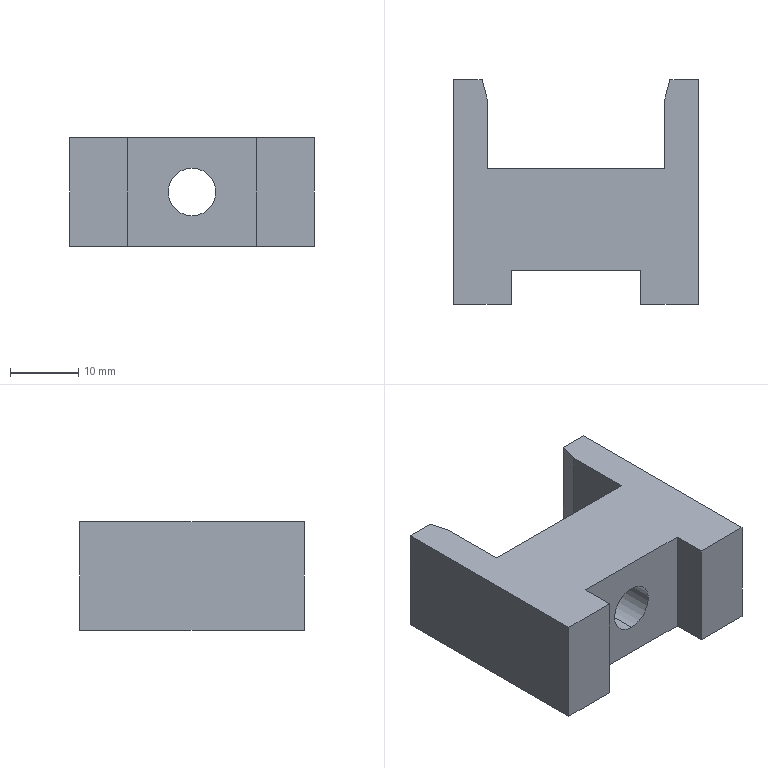Part | SolidWorks | features ICE 2, Extrusion 1 | 1 solid | 21 faces | box 36 x 33 x 16 mm | volume 11068 mm3 | plane 17 | cylinder 4 | commonest cylinder face diameters 7 x2 11 x2
STEP:
#1=CARTESIAN_POINT('',(18.,5.,4.5));
#2=VERTEX_POINT('',#1);
#3=CARTESIAN_POINT('',(18.,5.,11.5));
#4=VERTEX_POINT('',#3);
#5=CARTESIAN_POINT('',(18.,5.,8.));
#6=DIRECTION('',(0.,1.,0.));
#7=DIRECTION('',(0.,0.,1.));
#8=AXIS2_PLACEMENT_3D('',#5,#6,#7);
#9=CIRCLE('',#8,3.5);
#10=EDGE_CURVE('',#2,#4,#9,.T.);
#11=ORIENTED_EDGE('',*,*,#10,.F.);
#12=CARTESIAN_POINT('',(18.,13.,4.5));
#13=VERTEX_POINT('',#12);
#14=CARTESIAN_POINT('',(18.,5.,4.5));
#15=DIRECTION('',(0.,1.,0.));
#16=VECTOR('',#15,1000.);
#17=LINE('',#14,#16);
#18=EDGE_CURVE('',#2,#13,#17,.T.);
#19=ORIENTED_EDGE('',*,*,#18,.T.);
#20=CARTESIAN_POINT('',(18.,13.,11.5));
#21=VERTEX_POINT('',#20);
#22=CARTESIAN_POINT('',(18.,13.,8.));
#23=DIRECTION('',(0.,1.,0.));
#24=DIRECTION('',(0.,0.,1.));
#25=AXIS2_PLACEMENT_3D('',#22,#23,#24);
#26=CIRCLE('',#25,3.5);
#27=EDGE_CURVE('',#13,#21,#26,.T.);
#28=ORIENTED_EDGE('',*,*,#27,.T.);
#29=CARTESIAN_POINT('',(18.,5.,11.5));
#30=DIRECTION('',(0.,1.,0.));
#31=VECTOR('',#30,1000.);
#32=LINE('',#29,#31);
#33=EDGE_CURVE('',#4,#21,#32,.T.);
#34=ORIENTED_EDGE('',*,*,#33,.F.);
#35=EDGE_LOOP('',(#11,#19,#28,#34));
#36=FACE_OUTER_BOUND('',#35,.T.);
#37=CARTESIAN_POINT('',(18.,5.,8.));
#38=DIRECTION('',(0.,1.,0.));
#39=DIRECTION('',(0.,0.,1.));
#40=AXIS2_PLACEMENT_3D('',#37,#38,#39);
#41=CYLINDRICAL_SURFACE('',#40,3.5);
#42=ADVANCED_FACE('',(#36),#41,.F.);
#43=CARTESIAN_POINT('',(18.,13.,2.5));
#44=VERTEX_POINT('',#43);
#45=CARTESIAN_POINT('',(18.,13.,13.5));
#46=VERTEX_POINT('',#45);
#47=CARTESIAN_POINT('',(18.,13.,8.));
#48=DIRECTION('',(0.,1.,0.));
#49=DIRECTION('',(0.,0.,1.));
#50=AXIS2_PLACEMENT_3D('',#47,#48,#49);
#51=CIRCLE('',#50,5.5);
#52=EDGE_CURVE('',#44,#46,#51,.T.);
#53=ORIENTED_EDGE('',*,*,#52,.F.);
#54=CARTESIAN_POINT('',(18.,20.,2.5));
#55=VERTEX_POINT('',#54);
#56=CARTESIAN_POINT('',(18.,13.,2.5));
#57=DIRECTION('',(0.,1.,0.));
#58=VECTOR('',#57,1000.);
#59=LINE('',#56,#58);
#60=EDGE_CURVE('',#44,#55,#59,.T.);
#61=ORIENTED_EDGE('',*,*,#60,.T.);
#62=CARTESIAN_POINT('',(18.,20.,13.5));
#63=VERTEX_POINT('',#62);
#64=CARTESIAN_POINT('',(18.,20.,8.));
#65=DIRECTION('',(0.,1.,0.));
#66=DIRECTION('',(0.,0.,1.));
#67=AXIS2_PLACEMENT_3D('',#64,#65,#66);
#68=CIRCLE('',#67,5.5);
#69=EDGE_CURVE('',#55,#63,#68,.T.);
#70=ORIENTED_EDGE('',*,*,#69,.T.);
#71=CARTESIAN_POINT('',(18.,13.,13.5));
#72=DIRECTION('',(0.,1.,0.));
#73=VECTOR('',#72,1000.);
#74=LINE('',#71,#73);
#75=EDGE_CURVE('',#46,#63,#74,.T.);
#76=ORIENTED_EDGE('',*,*,#75,.F.);
#77=EDGE_LOOP('',(#53,#61,#70,#76));
#78=FACE_OUTER_BOUND('',#77,.T.);
#79=CARTESIAN_POINT('',(18.,13.,8.));
#80=DIRECTION('',(0.,1.,0.));
#81=DIRECTION('',(0.,0.,1.));
#82=AXIS2_PLACEMENT_3D('',#79,#80,#81);
#83=CYLINDRICAL_SURFACE('',#82,5.5);
#84=ADVANCED_FACE('',(#78),#83,.F.);
#85=CARTESIAN_POINT('',(4.196,33.,0.));
#86=VERTEX_POINT('',#85);
#87=CARTESIAN_POINT('',(0.,33.,0.));
#88=VERTEX_POINT('',#87);
#89=CARTESIAN_POINT('',(0.,33.,0.));
#90=DIRECTION('',(-1.,0.,0.));
#91=VECTOR('',#90,1000.);
#92=LINE('',#89,#91);
#93=EDGE_CURVE('',#86,#88,#92,.T.);
#94=ORIENTED_EDGE('',*,*,#93,.T.);
#95=CARTESIAN_POINT('',(0.,33.,16.));
#96=VERTEX_POINT('',#95);
#97=CARTESIAN_POINT('',(0.,33.,16.));
#98=DIRECTION('',(0.,0.,-1.));
#99=VECTOR('',#98,1000.);
#100=LINE('',#97,#99);
#101=EDGE_CURVE('',#96,#88,#100,.T.);
#102=ORIENTED_EDGE('',*,*,#101,.F.);
#103=CARTESIAN_POINT('',(4.196,33.,16.));
#104=VERTEX_POINT('',#103);
#105=CARTESIAN_POINT('',(0.,33.,16.));
#106=DIRECTION('',(-1.,0.,0.));
#107=VECTOR('',#106,1000.);
#108=LINE('',#105,#107);
#109=EDGE_CURVE('',#104,#96,#108,.T.);
#110=ORIENTED_EDGE('',*,*,#109,.F.);
#111=CARTESIAN_POINT('',(4.196,33.,16.));
#112=DIRECTION('',(0.,0.,-1.));
#113=VECTOR('',#112,1000.);
#114=LINE('',#111,#113);
#115=EDGE_CURVE('',#104,#86,#114,.T.);
#116=ORIENTED_EDGE('',*,*,#115,.T.);
#117=EDGE_LOOP('',(#94,#102,#110,#116));
#118=FACE_OUTER_BOUND('',#117,.T.);
#119=CARTESIAN_POINT('',(0.,33.,16.));
#120=DIRECTION('',(0.,-1.,0.));
#121=DIRECTION('',(0.,0.,-1.));
#122=AXIS2_PLACEMENT_3D('',#119,#120,#121);
#123=PLANE('',#122);
#124=ADVANCED_FACE('',(#118),#123,.F.);
#125=CARTESIAN_POINT('',(0.,0.,0.));
#126=VERTEX_POINT('',#125);
#127=CARTESIAN_POINT('',(0.,33.,0.));
#128=DIRECTION('',(0.,-1.,0.));
#129=VECTOR('',#128,1000.);
#130=LINE('',#127,#129);
#131=EDGE_CURVE('',#88,#126,#130,.T.);
#132=ORIENTED_EDGE('',*,*,#131,.T.);
#133=CARTESIAN_POINT('',(0.,0.,16.));
#134=VERTEX_POINT('',#133);
#135=CARTESIAN_POINT('',(0.,0.,16.));
#136=DIRECTION('',(0.,0.,-1.));
#137=VECTOR('',#136,1000.);
#138=LINE('',#135,#137);
#139=EDGE_CURVE('',#134,#126,#138,.T.);
#140=ORIENTED_EDGE('',*,*,#139,.F.);
#141=CARTESIAN_POINT('',(0.,33.,16.));
#142=DIRECTION('',(0.,-1.,0.));
#143=VECTOR('',#142,1000.);
#144=LINE('',#141,#143);
#145=EDGE_CURVE('',#96,#134,#144,.T.);
#146=ORIENTED_EDGE('',*,*,#145,.F.);
#147=ORIENTED_EDGE('',*,*,#101,.T.);
#148=EDGE_LOOP('',(#132,#140,#146,#147));
#149=FACE_OUTER_BOUND('',#148,.T.);
#150=CARTESIAN_POINT('',(0.,33.,16.));
#151=DIRECTION('',(1.,0.,0.));
#152=DIRECTION('',(0.,0.,-1.));
#153=AXIS2_PLACEMENT_3D('',#150,#151,#152);
#154=PLANE('',#153);
#155=ADVANCED_FACE('',(#149),#154,.F.);
#156=CARTESIAN_POINT('',(8.5,0.,0.));
#157=VERTEX_POINT('',#156);
#158=CARTESIAN_POINT('',(0.,0.,0.));
#159=DIRECTION('',(1.,0.,0.));
#160=VECTOR('',#159,1000.);
#161=LINE('',#158,#160);
#162=EDGE_CURVE('',#126,#157,#161,.T.);
#163=ORIENTED_EDGE('',*,*,#162,.T.);
#164=CARTESIAN_POINT('',(8.5,0.,16.));
#165=VERTEX_POINT('',#164);
#166=CARTESIAN_POINT('',(8.5,0.,16.));
#167=DIRECTION('',(0.,0.,-1.));
#168=VECTOR('',#167,1000.);
#169=LINE('',#166,#168);
#170=EDGE_CURVE('',#165,#157,#169,.T.);
#171=ORIENTED_EDGE('',*,*,#170,.F.);
#172=CARTESIAN_POINT('',(0.,0.,16.));
#173=DIRECTION('',(1.,0.,0.));
#174=VECTOR('',#173,1000.);
#175=LINE('',#172,#174);
#176=EDGE_CURVE('',#134,#165,#175,.T.);
#177=ORIENTED_EDGE('',*,*,#176,.F.);
#178=ORIENTED_EDGE('',*,*,#139,.T.);
#179=EDGE_LOOP('',(#163,#171,#177,#178));
#180=FACE_OUTER_BOUND('',#179,.T.);
#181=CARTESIAN_POINT('',(0.,0.,16.));
#182=DIRECTION('',(0.,1.,0.));
#183=DIRECTION('',(0.,0.,1.));
#184=AXIS2_PLACEMENT_3D('',#181,#182,#183);
#185=PLANE('',#184);
#186=ADVANCED_FACE('',(#180),#185,.F.);
#187=CARTESIAN_POINT('',(8.5,5.,0.));
#188=VERTEX_POINT('',#187);
#189=CARTESIAN_POINT('',(8.5,0.,0.));
#190=DIRECTION('',(0.,1.,0.));
#191=VECTOR('',#190,1000.);
#192=LINE('',#189,#191);
#193=EDGE_CURVE('',#157,#188,#192,.T.);
#194=ORIENTED_EDGE('',*,*,#193,.T.);
#195=CARTESIAN_POINT('',(8.5,5.,16.));
#196=VERTEX_POINT('',#195);
#197=CARTESIAN_POINT('',(8.5,5.,16.));
#198=DIRECTION('',(0.,0.,-1.));
#199=VECTOR('',#198,1000.);
#200=LINE('',#197,#199);
#201=EDGE_CURVE('',#196,#188,#200,.T.);
#202=ORIENTED_EDGE('',*,*,#201,.F.);
#203=CARTESIAN_POINT('',(8.5,0.,16.));
#204=DIRECTION('',(0.,1.,0.));
#205=VECTOR('',#204,1000.);
#206=LINE('',#203,#205);
#207=EDGE_CURVE('',#165,#196,#206,.T.);
#208=ORIENTED_EDGE('',*,*,#207,.F.);
#209=ORIENTED_EDGE('',*,*,#170,.T.);
#210=EDGE_LOOP('',(#194,#202,#208,#209));
#211=FACE_OUTER_BOUND('',#210,.T.);
#212=CARTESIAN_POINT('',(8.5,0.,16.));
#213=DIRECTION('',(-1.,0.,0.));
#214=DIRECTION('',(0.,0.,1.));
#215=AXIS2_PLACEMENT_3D('',#212,#213,#214);
#216=PLANE('',#215);
#217=ADVANCED_FACE('',(#211),#216,.F.);
#218=CARTESIAN_POINT('',(18.,5.,8.));
#219=DIRECTION('',(0.,1.,0.));
#220=DIRECTION('',(0.,0.,1.));
#221=AXIS2_PLACEMENT_3D('',#218,#219,#220);
#222=CIRCLE('',#221,3.5);
#223=EDGE_CURVE('',#4,#2,#222,.T.);
#224=ORIENTED_EDGE('',*,*,#223,.T.);
#225=ORIENTED_EDGE('',*,*,#10,.T.);
#226=EDGE_LOOP('',(#224,#225));
#227=FACE_BOUND('',#226,.T.);
#228=CARTESIAN_POINT('',(27.5,5.,0.));
#229=VERTEX_POINT('',#228);
#230=CARTESIAN_POINT('',(8.5,5.,0.));
#231=DIRECTION('',(1.,0.,0.));
#232=VECTOR('',#231,1000.);
#233=LINE('',#230,#232);
#234=EDGE_CURVE('',#188,#229,#233,.T.);
#235=ORIENTED_EDGE('',*,*,#234,.T.);
#236=CARTESIAN_POINT('',(27.5,5.,16.));
#237=VERTEX_POINT('',#236);
#238=CARTESIAN_POINT('',(27.5,5.,16.));
#239=DIRECTION('',(0.,0.,-1.));
#240=VECTOR('',#239,1000.);
#241=LINE('',#238,#240);
#242=EDGE_CURVE('',#237,#229,#241,.T.);
#243=ORIENTED_EDGE('',*,*,#242,.F.);
#244=CARTESIAN_POINT('',(8.5,5.,16.));
#245=DIRECTION('',(1.,0.,0.));
#246=VECTOR('',#245,1000.);
#247=LINE('',#244,#246);
#248=EDGE_CURVE('',#196,#237,#247,.T.);
#249=ORIENTED_EDGE('',*,*,#248,.F.);
#250=ORIENTED_EDGE('',*,*,#201,.T.);
#251=EDGE_LOOP('',(#235,#243,#249,#250));
#252=FACE_OUTER_BOUND('',#251,.T.);
#253=CARTESIAN_POINT('',(8.5,5.,16.));
#254=DIRECTION('',(0.,1.,0.));
#255=DIRECTION('',(0.,0.,1.));
#256=AXIS2_PLACEMENT_3D('',#253,#254,#255);
#257=PLANE('',#256);
#258=ADVANCED_FACE('',(#227,#252),#257,.F.);
#259=CARTESIAN_POINT('',(27.5,0.,0.));
#260=VERTEX_POINT('',#259);
#261=CARTESIAN_POINT('',(27.5,5.,0.));
#262=DIRECTION('',(0.,-1.,0.));
#263=VECTOR('',#262,1000.);
#264=LINE('',#261,#263);
#265=EDGE_CURVE('',#229,#260,#264,.T.);
#266=ORIENTED_EDGE('',*,*,#265,.T.);
#267=CARTESIAN_POINT('',(27.5,0.,16.));
#268=VERTEX_POINT('',#267);
#269=CARTESIAN_POINT('',(27.5,0.,16.));
#270=DIRECTION('',(0.,0.,-1.));
#271=VECTOR('',#270,1000.);
#272=LINE('',#269,#271);
#273=EDGE_CURVE('',#268,#260,#272,.T.);
#274=ORIENTED_EDGE('',*,*,#273,.F.);
#275=CARTESIAN_POINT('',(27.5,5.,16.));
#276=DIRECTION('',(0.,-1.,0.));
#277=VECTOR('',#276,1000.);
#278=LINE('',#275,#277);
#279=EDGE_CURVE('',#237,#268,#278,.T.);
#280=ORIENTED_EDGE('',*,*,#279,.F.);
#281=ORIENTED_EDGE('',*,*,#242,.T.);
#282=EDGE_LOOP('',(#266,#274,#280,#281));
#283=FACE_OUTER_BOUND('',#282,.T.);
#284=CARTESIAN_POINT('',(27.5,5.,16.));
#285=DIRECTION('',(1.,0.,0.));
#286=DIRECTION('',(0.,0.,-1.));
#287=AXIS2_PLACEMENT_3D('',#284,#285,#286);
#288=PLANE('',#287);
#289=ADVANCED_FACE('',(#283),#288,.F.);
#290=CARTESIAN_POINT('',(36.,0.,0.));
#291=VERTEX_POINT('',#290);
#292=CARTESIAN_POINT('',(27.5,0.,0.));
#293=DIRECTION('',(1.,0.,0.));
#294=VECTOR('',#293,1000.);
#295=LINE('',#292,#294);
#296=EDGE_CURVE('',#260,#291,#295,.T.);
#297=ORIENTED_EDGE('',*,*,#296,.T.);
#298=CARTESIAN_POINT('',(36.,0.,16.));
#299=VERTEX_POINT('',#298);
#300=CARTESIAN_POINT('',(36.,0.,16.));
#301=DIRECTION('',(0.,0.,-1.));
#302=VECTOR('',#301,1000.);
#303=LINE('',#300,#302);
#304=EDGE_CURVE('',#299,#291,#303,.T.);
#305=ORIENTED_EDGE('',*,*,#304,.F.);
#306=CARTESIAN_POINT('',(27.5,0.,16.));
#307=DIRECTION('',(1.,0.,0.));
#308=VECTOR('',#307,1000.);
#309=LINE('',#306,#308);
#310=EDGE_CURVE('',#268,#299,#309,.T.);
#311=ORIENTED_EDGE('',*,*,#310,.F.);
#312=ORIENTED_EDGE('',*,*,#273,.T.);
#313=EDGE_LOOP('',(#297,#305,#311,#312));
#314=FACE_OUTER_BOUND('',#313,.T.);
#315=CARTESIAN_POINT('',(27.5,0.,16.));
#316=DIRECTION('',(0.,1.,0.));
#317=DIRECTION('',(0.,0.,1.));
#318=AXIS2_PLACEMENT_3D('',#315,#316,#317);
#319=PLANE('',#318);
#320=ADVANCED_FACE('',(#314),#319,.F.);
#321=CARTESIAN_POINT('',(36.,33.,0.));
#322=VERTEX_POINT('',#321);
#323=CARTESIAN_POINT('',(36.,0.,0.));
#324=DIRECTION('',(0.,1.,0.));
#325=VECTOR('',#324,1000.);
#326=LINE('',#323,#325);
#327=EDGE_CURVE('',#291,#322,#326,.T.);
#328=ORIENTED_EDGE('',*,*,#327,.T.);
#329=CARTESIAN_POINT('',(36.,33.,16.));
#330=VERTEX_POINT('',#329);
#331=CARTESIAN_POINT('',(36.,33.,16.));
#332=DIRECTION('',(0.,0.,-1.));
#333=VECTOR('',#332,1000.);
#334=LINE('',#331,#333);
#335=EDGE_CURVE('',#330,#322,#334,.T.);
#336=ORIENTED_EDGE('',*,*,#335,.F.);
#337=CARTESIAN_POINT('',(36.,0.,16.));
#338=DIRECTION('',(0.,1.,0.));
#339=VECTOR('',#338,1000.);
#340=LINE('',#337,#339);
#341=EDGE_CURVE('',#299,#330,#340,.T.);
#342=ORIENTED_EDGE('',*,*,#341,.F.);
#343=ORIENTED_EDGE('',*,*,#304,.T.);
#344=EDGE_LOOP('',(#328,#336,#342,#343));
#345=FACE_OUTER_BOUND('',#344,.T.);
#346=CARTESIAN_POINT('',(36.,0.,16.));
#347=DIRECTION('',(-1.,0.,0.));
#348=DIRECTION('',(0.,0.,1.));
#349=AXIS2_PLACEMENT_3D('',#346,#347,#348);
#350=PLANE('',#349);
#351=ADVANCED_FACE('',(#345),#350,.F.);
#352=CARTESIAN_POINT('',(31.804,33.,0.));
#353=VERTEX_POINT('',#352);
#354=CARTESIAN_POINT('',(31.804,33.,0.));
#355=DIRECTION('',(-1.,0.,0.));
#356=VECTOR('',#355,1000.);
#357=LINE('',#354,#356);
#358=EDGE_CURVE('',#322,#353,#357,.T.);
#359=ORIENTED_EDGE('',*,*,#358,.T.);
#360=CARTESIAN_POINT('',(31.804,33.,16.));
#361=VERTEX_POINT('',#360);
#362=CARTESIAN_POINT('',(31.804,33.,16.));
#363=DIRECTION('',(0.,0.,-1.));
#364=VECTOR('',#363,1000.);
#365=LINE('',#362,#364);
#366=EDGE_CURVE('',#361,#353,#365,.T.);
#367=ORIENTED_EDGE('',*,*,#366,.F.);
#368=CARTESIAN_POINT('',(31.804,33.,16.));
#369=DIRECTION('',(-1.,0.,0.));
#370=VECTOR('',#369,1000.);
#371=LINE('',#368,#370);
#372=EDGE_CURVE('',#330,#361,#371,.T.);
#373=ORIENTED_EDGE('',*,*,#372,.F.);
#374=ORIENTED_EDGE('',*,*,#335,.T.);
#375=EDGE_LOOP('',(#359,#367,#373,#374));
#376=FACE_OUTER_BOUND('',#375,.T.);
#377=CARTESIAN_POINT('',(31.804,33.,16.));
#378=DIRECTION('',(0.,-1.,0.));
#379=DIRECTION('',(0.,0.,-1.));
#380=AXIS2_PLACEMENT_3D('',#377,#378,#379);
#381=PLANE('',#380);
#382=ADVANCED_FACE('',(#376),#381,.F.);
#383=CARTESIAN_POINT('',(31.,30.,0.));
#384=VERTEX_POINT('',#383);
#385=CARTESIAN_POINT('',(31.,30.,0.));
#386=DIRECTION('',(-0.2588,-0.9659,0.));
#387=VECTOR('',#386,1000.);
#388=LINE('',#385,#387);
#389=EDGE_CURVE('',#353,#384,#388,.T.);
#390=ORIENTED_EDGE('',*,*,#389,.T.);
#391=CARTESIAN_POINT('',(31.,30.,16.));
#392=VERTEX_POINT('',#391);
#393=CARTESIAN_POINT('',(31.,30.,16.));
#394=DIRECTION('',(0.,0.,-1.));
#395=VECTOR('',#394,1000.);
#396=LINE('',#393,#395);
#397=EDGE_CURVE('',#392,#384,#396,.T.);
#398=ORIENTED_EDGE('',*,*,#397,.F.);
#399=CARTESIAN_POINT('',(31.,30.,16.));
#400=DIRECTION('',(-0.2588,-0.9659,0.));
#401=VECTOR('',#400,1000.);
#402=LINE('',#399,#401);
#403=EDGE_CURVE('',#361,#392,#402,.T.);
#404=ORIENTED_EDGE('',*,*,#403,.F.);
#405=ORIENTED_EDGE('',*,*,#366,.T.);
#406=EDGE_LOOP('',(#390,#398,#404,#405));
#407=FACE_OUTER_BOUND('',#406,.T.);
#408=CARTESIAN_POINT('',(31.,30.,16.));
#409=DIRECTION('',(0.9659,-0.2588,0.));
#410=DIRECTION('',(0.2588,0.9659,0.));
#411=AXIS2_PLACEMENT_3D('',#408,#409,#410);
#412=PLANE('',#411);
#413=ADVANCED_FACE('',(#407),#412,.F.);
#414=CARTESIAN_POINT('',(31.,20.,0.));
#415=VERTEX_POINT('',#414);
#416=CARTESIAN_POINT('',(31.,20.,0.));
#417=DIRECTION('',(0.,-1.,0.));
#418=VECTOR('',#417,1000.);
#419=LINE('',#416,#418);
#420=EDGE_CURVE('',#384,#415,#419,.T.);
#421=ORIENTED_EDGE('',*,*,#420,.T.);
#422=CARTESIAN_POINT('',(31.,20.,16.));
#423=VERTEX_POINT('',#422);
#424=CARTESIAN_POINT('',(31.,20.,16.));
#425=DIRECTION('',(0.,0.,-1.));
#426=VECTOR('',#425,1000.);
#427=LINE('',#424,#426);
#428=EDGE_CURVE('',#423,#415,#427,.T.);
#429=ORIENTED_EDGE('',*,*,#428,.F.);
#430=CARTESIAN_POINT('',(31.,20.,16.));
#431=DIRECTION('',(0.,-1.,0.));
#432=VECTOR('',#431,1000.);
#433=LINE('',#430,#432);
#434=EDGE_CURVE('',#392,#423,#433,.T.);
#435=ORIENTED_EDGE('',*,*,#434,.F.);
#436=ORIENTED_EDGE('',*,*,#397,.T.);
#437=EDGE_LOOP('',(#421,#429,#435,#436));
#438=FACE_OUTER_BOUND('',#437,.T.);
#439=CARTESIAN_POINT('',(31.,20.,16.));
#440=DIRECTION('',(1.,0.,0.));
#441=DIRECTION('',(0.,0.,-1.));
#442=AXIS2_PLACEMENT_3D('',#439,#440,#441);
#443=PLANE('',#442);
#444=ADVANCED_FACE('',(#438),#443,.F.);
#445=CARTESIAN_POINT('',(18.,20.,8.));
#446=DIRECTION('',(0.,1.,0.));
#447=DIRECTION('',(0.,0.,1.));
#448=AXIS2_PLACEMENT_3D('',#445,#446,#447);
#449=CIRCLE('',#448,5.5);
#450=EDGE_CURVE('',#63,#55,#449,.T.);
#451=ORIENTED_EDGE('',*,*,#450,.F.);
#452=ORIENTED_EDGE('',*,*,#69,.F.);
#453=EDGE_LOOP('',(#451,#452));
#454=FACE_BOUND('',#453,.T.);
#455=CARTESIAN_POINT('',(5.,20.,0.));
#456=VERTEX_POINT('',#455);
#457=CARTESIAN_POINT('',(5.,20.,0.));
#458=DIRECTION('',(-1.,0.,0.));
#459=VECTOR('',#458,1000.);
#460=LINE('',#457,#459);
#461=EDGE_CURVE('',#415,#456,#460,.T.);
#462=ORIENTED_EDGE('',*,*,#461,.T.);
#463=CARTESIAN_POINT('',(5.,20.,16.));
#464=VERTEX_POINT('',#463);
#465=CARTESIAN_POINT('',(5.,20.,16.));
#466=DIRECTION('',(0.,0.,-1.));
#467=VECTOR('',#466,1000.);
#468=LINE('',#465,#467);
#469=EDGE_CURVE('',#464,#456,#468,.T.);
#470=ORIENTED_EDGE('',*,*,#469,.F.);
#471=CARTESIAN_POINT('',(5.,20.,16.));
#472=DIRECTION('',(-1.,0.,0.));
#473=VECTOR('',#472,1000.);
#474=LINE('',#471,#473);
#475=EDGE_CURVE('',#423,#464,#474,.T.);
#476=ORIENTED_EDGE('',*,*,#475,.F.);
#477=ORIENTED_EDGE('',*,*,#428,.T.);
#478=EDGE_LOOP('',(#462,#470,#476,#477));
#479=FACE_OUTER_BOUND('',#478,.T.);
#480=CARTESIAN_POINT('',(5.,20.,16.));
#481=DIRECTION('',(0.,-1.,0.));
#482=DIRECTION('',(0.,0.,-1.));
#483=AXIS2_PLACEMENT_3D('',#480,#481,#482);
#484=PLANE('',#483);
#485=ADVANCED_FACE('',(#454,#479),#484,.F.);
#486=CARTESIAN_POINT('',(5.,30.,0.));
#487=VERTEX_POINT('',#486);
#488=CARTESIAN_POINT('',(5.,30.,0.));
#489=DIRECTION('',(0.,1.,0.));
#490=VECTOR('',#489,1000.);
#491=LINE('',#488,#490);
#492=EDGE_CURVE('',#456,#487,#491,.T.);
#493=ORIENTED_EDGE('',*,*,#492,.T.);
#494=CARTESIAN_POINT('',(5.,30.,16.));
#495=VERTEX_POINT('',#494);
#496=CARTESIAN_POINT('',(5.,30.,16.));
#497=DIRECTION('',(0.,0.,-1.));
#498=VECTOR('',#497,1000.);
#499=LINE('',#496,#498);
#500=EDGE_CURVE('',#495,#487,#499,.T.);
#501=ORIENTED_EDGE('',*,*,#500,.F.);
#502=CARTESIAN_POINT('',(5.,30.,16.));
#503=DIRECTION('',(0.,1.,0.));
#504=VECTOR('',#503,1000.);
#505=LINE('',#502,#504);
#506=EDGE_CURVE('',#464,#495,#505,.T.);
#507=ORIENTED_EDGE('',*,*,#506,.F.);
#508=ORIENTED_EDGE('',*,*,#469,.T.);
#509=EDGE_LOOP('',(#493,#501,#507,#508));
#510=FACE_OUTER_BOUND('',#509,.T.);
#511=CARTESIAN_POINT('',(5.,30.,16.));
#512=DIRECTION('',(-1.,0.,0.));
#513=DIRECTION('',(0.,-1.,0.));
#514=AXIS2_PLACEMENT_3D('',#511,#512,#513);
#515=PLANE('',#514);
#516=ADVANCED_FACE('',(#510),#515,.F.);
#517=CARTESIAN_POINT('',(4.196,33.,0.));
#518=DIRECTION('',(-0.2588,0.9659,0.));
#519=VECTOR('',#518,1000.);
#520=LINE('',#517,#519);
#521=EDGE_CURVE('',#487,#86,#520,.T.);
#522=ORIENTED_EDGE('',*,*,#521,.T.);
#523=ORIENTED_EDGE('',*,*,#115,.F.);
#524=CARTESIAN_POINT('',(4.196,33.,16.));
#525=DIRECTION('',(-0.2588,0.9659,0.));
#526=VECTOR('',#525,1000.);
#527=LINE('',#524,#526);
#528=EDGE_CURVE('',#495,#104,#527,.T.);
#529=ORIENTED_EDGE('',*,*,#528,.F.);
#530=ORIENTED_EDGE('',*,*,#500,.T.);
#531=EDGE_LOOP('',(#522,#523,#529,#530));
#532=FACE_OUTER_BOUND('',#531,.T.);
#533=CARTESIAN_POINT('',(4.196,33.,16.));
#534=DIRECTION('',(-0.9659,-0.2588,0.));
#535=DIRECTION('',(0.2588,-0.9659,0.));
#536=AXIS2_PLACEMENT_3D('',#533,#534,#535);
#537=PLANE('',#536);
#538=ADVANCED_FACE('',(#532),#537,.F.);
#539=ORIENTED_EDGE('',*,*,#109,.T.);
#540=ORIENTED_EDGE('',*,*,#145,.T.);
#541=ORIENTED_EDGE('',*,*,#176,.T.);
#542=ORIENTED_EDGE('',*,*,#207,.T.);
#543=ORIENTED_EDGE('',*,*,#248,.T.);
#544=ORIENTED_EDGE('',*,*,#279,.T.);
#545=ORIENTED_EDGE('',*,*,#310,.T.);
#546=ORIENTED_EDGE('',*,*,#341,.T.);
#547=ORIENTED_EDGE('',*,*,#372,.T.);
#548=ORIENTED_EDGE('',*,*,#403,.T.);
#549=ORIENTED_EDGE('',*,*,#434,.T.);
#550=ORIENTED_EDGE('',*,*,#475,.T.);
#551=ORIENTED_EDGE('',*,*,#506,.T.);
#552=ORIENTED_EDGE('',*,*,#528,.T.);
#553=EDGE_LOOP('',(#539,#540,#541,#542,#543,#544,#545,#546,#547,#548,#549,#550,#551,#552));
#554=FACE_OUTER_BOUND('',#553,.T.);
#555=CARTESIAN_POINT('',(0.,0.,16.));
#556=DIRECTION('',(0.,0.,-1.));
#557=DIRECTION('',(-1.,0.,0.));
#558=AXIS2_PLACEMENT_3D('',#555,#556,#557);
#559=PLANE('',#558);
#560=ADVANCED_FACE('',(#554),#559,.F.);
#561=ORIENTED_EDGE('',*,*,#93,.F.);
#562=ORIENTED_EDGE('',*,*,#521,.F.);
#563=ORIENTED_EDGE('',*,*,#492,.F.);
#564=ORIENTED_EDGE('',*,*,#461,.F.);
#565=ORIENTED_EDGE('',*,*,#420,.F.);
#566=ORIENTED_EDGE('',*,*,#389,.F.);
#567=ORIENTED_EDGE('',*,*,#358,.F.);
#568=ORIENTED_EDGE('',*,*,#327,.F.);
#569=ORIENTED_EDGE('',*,*,#296,.F.);
#570=ORIENTED_EDGE('',*,*,#265,.F.);
#571=ORIENTED_EDGE('',*,*,#234,.F.);
#572=ORIENTED_EDGE('',*,*,#193,.F.);
#573=ORIENTED_EDGE('',*,*,#162,.F.);
#574=ORIENTED_EDGE('',*,*,#131,.F.);
#575=EDGE_LOOP('',(#561,#562,#563,#564,#565,#566,#567,#568,#569,#570,#571,#572,#573,#574));
#576=FACE_OUTER_BOUND('',#575,.T.);
#577=CARTESIAN_POINT('',(0.,0.,0.));
#578=DIRECTION('',(0.,0.,-1.));
#579=DIRECTION('',(-1.,0.,0.));
#580=AXIS2_PLACEMENT_3D('',#577,#578,#579);
#581=PLANE('',#580);
#582=ADVANCED_FACE('',(#576),#581,.T.);
#583=ORIENTED_EDGE('',*,*,#60,.F.);
#584=CARTESIAN_POINT('',(18.,13.,8.));
#585=DIRECTION('',(0.,1.,0.));
#586=DIRECTION('',(0.,0.,1.));
#587=AXIS2_PLACEMENT_3D('',#584,#585,#586);
#588=CIRCLE('',#587,5.5);
#589=EDGE_CURVE('',#46,#44,#588,.T.);
#590=ORIENTED_EDGE('',*,*,#589,.F.);
#591=ORIENTED_EDGE('',*,*,#75,.T.);
#592=ORIENTED_EDGE('',*,*,#450,.T.);
#593=EDGE_LOOP('',(#583,#590,#591,#592));
#594=FACE_OUTER_BOUND('',#593,.T.);
#595=CARTESIAN_POINT('',(18.,13.,8.));
#596=DIRECTION('',(0.,1.,0.));
#597=DIRECTION('',(0.,0.,1.));
#598=AXIS2_PLACEMENT_3D('',#595,#596,#597);
#599=CYLINDRICAL_SURFACE('',#598,5.5);
#600=ADVANCED_FACE('',(#594),#599,.F.);
#601=CARTESIAN_POINT('',(18.,13.,8.));
#602=DIRECTION('',(0.,1.,0.));
#603=DIRECTION('',(0.,0.,1.));
#604=AXIS2_PLACEMENT_3D('',#601,#602,#603);
#605=CIRCLE('',#604,3.5);
#606=EDGE_CURVE('',#21,#13,#605,.T.);
#607=ORIENTED_EDGE('',*,*,#606,.F.);
#608=ORIENTED_EDGE('',*,*,#27,.F.);
#609=EDGE_LOOP('',(#607,#608));
#610=FACE_BOUND('',#609,.T.);
#611=ORIENTED_EDGE('',*,*,#589,.T.);
#612=ORIENTED_EDGE('',*,*,#52,.T.);
#613=EDGE_LOOP('',(#611,#612));
#614=FACE_OUTER_BOUND('',#613,.T.);
#615=CARTESIAN_POINT('',(18.,13.,8.));
#616=DIRECTION('',(0.,1.,0.));
#617=DIRECTION('',(0.,0.,1.));
#618=AXIS2_PLACEMENT_3D('',#615,#616,#617);
#619=PLANE('',#618);
#620=ADVANCED_FACE('',(#610,#614),#619,.T.);
#621=ORIENTED_EDGE('',*,*,#18,.F.);
#622=ORIENTED_EDGE('',*,*,#223,.F.);
#623=ORIENTED_EDGE('',*,*,#33,.T.);
#624=ORIENTED_EDGE('',*,*,#606,.T.);
#625=EDGE_LOOP('',(#621,#622,#623,#624));
#626=FACE_OUTER_BOUND('',#625,.T.);
#627=CARTESIAN_POINT('',(18.,5.,8.));
#628=DIRECTION('',(0.,1.,0.));
#629=DIRECTION('',(0.,0.,1.));
#630=AXIS2_PLACEMENT_3D('',#627,#628,#629);
#631=CYLINDRICAL_SURFACE('',#630,3.5);
#632=ADVANCED_FACE('',(#626),#631,.F.);
#633=CLOSED_SHELL('',(#42,#84,#124,#155,#186,#217,#258,#289,#320,#351,#382,#413,#444,#485,#516,#538,#560,#582,#600,#620,#632));
#634=MANIFOLD_SOLID_BREP('',#633);
#635=CARTESIAN_POINT('',(0.,0.,0.));
#636=DIRECTION('',(0.,0.,1.));
#637=DIRECTION('',(1.,0.,0.));
#638=AXIS2_PLACEMENT_3D('',#635,#636,#637);
#639=(LENGTH_UNIT()NAMED_UNIT(*)SI_UNIT(.MILLI.,.METRE.));
#640=UNCERTAINTY_MEASURE_WITH_UNIT(LENGTH_MEASURE(0.00001),#639,'','');
#641=(NAMED_UNIT(*)PLANE_ANGLE_UNIT()SI_UNIT($,.RADIAN.));
#642=(NAMED_UNIT(*)SI_UNIT($,.STERADIAN.)SOLID_ANGLE_UNIT());
#643=(GEOMETRIC_REPRESENTATION_CONTEXT(3)GLOBAL_UNCERTAINTY_ASSIGNED_CONTEXT((#640))GLOBAL_UNIT_ASSIGNED_CONTEXT((#639,#641,#642))REPRESENTATION_CONTEXT('',''));
#644=ADVANCED_BREP_SHAPE_REPRESENTATION('',(#634,#638),#643);